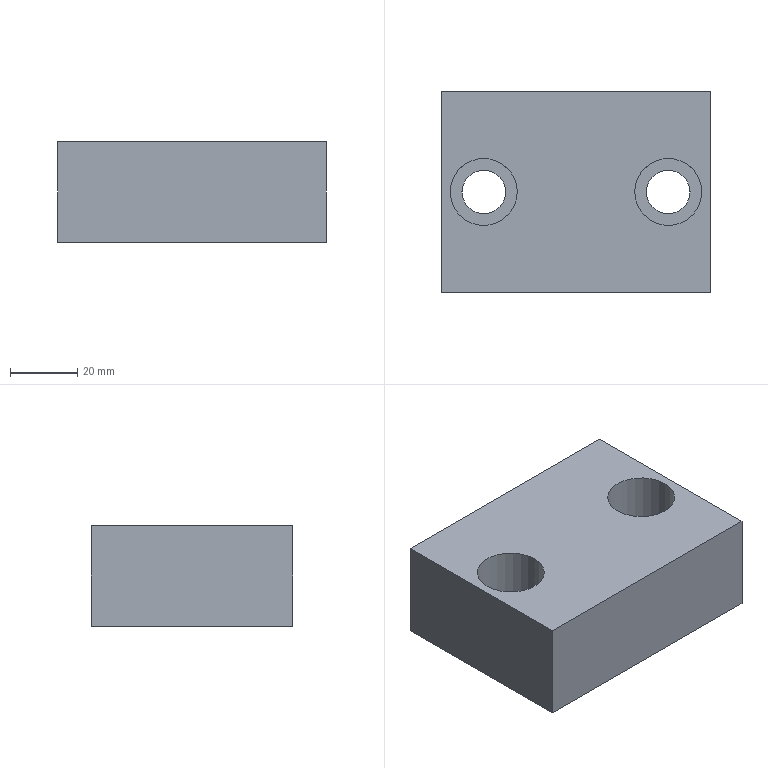Part | NX | features solid 2 | 1 solid | 12 faces | box 80 x 60 x 30 mm | volume 130956 mm3 | plane 8 | cylinder 4 | commonest cylinder face diameters 13 x2 20 x2
STEP:
#1=CARTESIAN_POINT('',(955.,365.,2.));
#2=VERTEX_POINT('',#1);
#3=CARTESIAN_POINT('',(955.,425.,2.));
#4=VERTEX_POINT('',#3);
#5=CARTESIAN_POINT('',(955.,365.,2.));
#6=DIRECTION('',(0.,1.,0.));
#7=VECTOR('',#6,1000.);
#8=LINE('',#5,#7);
#9=EDGE_CURVE('',#2,#4,#8,.T.);
#10=ORIENTED_EDGE('',*,*,#9,.F.);
#11=CARTESIAN_POINT('',(1035.,365.,2.));
#12=VERTEX_POINT('',#11);
#13=CARTESIAN_POINT('',(1035.,365.,2.));
#14=DIRECTION('',(-1.,0.,0.));
#15=VECTOR('',#14,1000.);
#16=LINE('',#13,#15);
#17=EDGE_CURVE('',#12,#2,#16,.T.);
#18=ORIENTED_EDGE('',*,*,#17,.F.);
#19=CARTESIAN_POINT('',(1035.,425.,2.));
#20=VERTEX_POINT('',#19);
#21=CARTESIAN_POINT('',(1035.,425.,2.));
#22=DIRECTION('',(0.,-1.,0.));
#23=VECTOR('',#22,1000.);
#24=LINE('',#21,#23);
#25=EDGE_CURVE('',#20,#12,#24,.T.);
#26=ORIENTED_EDGE('',*,*,#25,.F.);
#27=CARTESIAN_POINT('',(955.,425.,2.));
#28=DIRECTION('',(1.,0.,0.));
#29=VECTOR('',#28,1000.);
#30=LINE('',#27,#29);
#31=EDGE_CURVE('',#4,#20,#30,.T.);
#32=ORIENTED_EDGE('',*,*,#31,.F.);
#33=EDGE_LOOP('',(#10,#18,#26,#32));
#34=FACE_BOUND('',#33,.T.);
#35=CARTESIAN_POINT('',(1012.5,395.,2.));
#36=VERTEX_POINT('',#35);
#37=CARTESIAN_POINT('',(1022.5,395.,2.));
#38=DIRECTION('',(0.,0.,-1.));
#39=DIRECTION('',(-1.,0.,0.));
#40=AXIS2_PLACEMENT_3D('',#37,#38,#39);
#41=CIRCLE('',#40,10.);
#42=EDGE_CURVE('',#36,#36,#41,.T.);
#43=ORIENTED_EDGE('',*,*,#42,.T.);
#44=EDGE_LOOP('',(#43));
#45=FACE_BOUND('',#44,.T.);
#46=CARTESIAN_POINT('',(977.5,395.,2.));
#47=VERTEX_POINT('',#46);
#48=CARTESIAN_POINT('',(967.5,395.,2.));
#49=DIRECTION('',(0.,0.,1.));
#50=DIRECTION('',(1.,0.,0.));
#51=AXIS2_PLACEMENT_3D('',#48,#49,#50);
#52=CIRCLE('',#51,10.);
#53=EDGE_CURVE('',#47,#47,#52,.T.);
#54=ORIENTED_EDGE('',*,*,#53,.F.);
#55=EDGE_LOOP('',(#54));
#56=FACE_BOUND('',#55,.T.);
#57=CARTESIAN_POINT('',(955.,365.,2.));
#58=DIRECTION('',(0.,0.,1.));
#59=DIRECTION('',(1.,0.,0.));
#60=AXIS2_PLACEMENT_3D('',#57,#58,#59);
#61=PLANE('',#60);
#62=ADVANCED_FACE('',(#34,#45,#56),#61,.T.);
#63=CARTESIAN_POINT('',(974.,395.,-28.));
#64=VERTEX_POINT('',#63);
#65=CARTESIAN_POINT('',(967.5,395.,-28.));
#66=DIRECTION('',(0.,0.,1.));
#67=DIRECTION('',(1.,0.,0.));
#68=AXIS2_PLACEMENT_3D('',#65,#66,#67);
#69=CIRCLE('',#68,6.5);
#70=EDGE_CURVE('',#64,#64,#69,.T.);
#71=ORIENTED_EDGE('',*,*,#70,.F.);
#72=EDGE_LOOP('',(#71));
#73=FACE_BOUND('',#72,.T.);
#74=CARTESIAN_POINT('',(974.,395.,-12.));
#75=VERTEX_POINT('',#74);
#76=CARTESIAN_POINT('',(967.5,395.,-12.));
#77=DIRECTION('',(0.,0.,1.));
#78=DIRECTION('',(1.,0.,0.));
#79=AXIS2_PLACEMENT_3D('',#76,#77,#78);
#80=CIRCLE('',#79,6.5);
#81=EDGE_CURVE('',#75,#75,#80,.T.);
#82=ORIENTED_EDGE('',*,*,#81,.T.);
#83=EDGE_LOOP('',(#82));
#84=FACE_BOUND('',#83,.T.);
#85=CARTESIAN_POINT('',(967.5,395.,2.));
#86=DIRECTION('',(0.,0.,-1.));
#87=DIRECTION('',(-1.,0.,0.));
#88=AXIS2_PLACEMENT_3D('',#85,#86,#87);
#89=CYLINDRICAL_SURFACE('',#88,6.5);
#90=ADVANCED_FACE('',(#73,#84),#89,.F.);
#91=CARTESIAN_POINT('',(955.,365.,-28.));
#92=VERTEX_POINT('',#91);
#93=CARTESIAN_POINT('',(955.,425.,-28.));
#94=VERTEX_POINT('',#93);
#95=CARTESIAN_POINT('',(955.,365.,-28.));
#96=DIRECTION('',(0.,1.,0.));
#97=VECTOR('',#96,1000.);
#98=LINE('',#95,#97);
#99=EDGE_CURVE('',#92,#94,#98,.T.);
#100=ORIENTED_EDGE('',*,*,#99,.T.);
#101=CARTESIAN_POINT('',(1035.,425.,-28.));
#102=VERTEX_POINT('',#101);
#103=CARTESIAN_POINT('',(955.,425.,-28.));
#104=DIRECTION('',(1.,0.,0.));
#105=VECTOR('',#104,1000.);
#106=LINE('',#103,#105);
#107=EDGE_CURVE('',#94,#102,#106,.T.);
#108=ORIENTED_EDGE('',*,*,#107,.T.);
#109=CARTESIAN_POINT('',(1035.,365.,-28.));
#110=VERTEX_POINT('',#109);
#111=CARTESIAN_POINT('',(1035.,425.,-28.));
#112=DIRECTION('',(0.,-1.,0.));
#113=VECTOR('',#112,1000.);
#114=LINE('',#111,#113);
#115=EDGE_CURVE('',#102,#110,#114,.T.);
#116=ORIENTED_EDGE('',*,*,#115,.T.);
#117=CARTESIAN_POINT('',(1035.,365.,-28.));
#118=DIRECTION('',(-1.,0.,0.));
#119=VECTOR('',#118,1000.);
#120=LINE('',#117,#119);
#121=EDGE_CURVE('',#110,#92,#120,.T.);
#122=ORIENTED_EDGE('',*,*,#121,.T.);
#123=EDGE_LOOP('',(#100,#108,#116,#122));
#124=FACE_BOUND('',#123,.T.);
#125=CARTESIAN_POINT('',(1029.,395.,-28.));
#126=VERTEX_POINT('',#125);
#127=CARTESIAN_POINT('',(1022.5,395.,-28.));
#128=DIRECTION('',(0.,0.,1.));
#129=DIRECTION('',(1.,0.,0.));
#130=AXIS2_PLACEMENT_3D('',#127,#128,#129);
#131=CIRCLE('',#130,6.5);
#132=EDGE_CURVE('',#126,#126,#131,.F.);
#133=ORIENTED_EDGE('',*,*,#132,.F.);
#134=EDGE_LOOP('',(#133));
#135=FACE_BOUND('',#134,.T.);
#136=ORIENTED_EDGE('',*,*,#70,.T.);
#137=EDGE_LOOP('',(#136));
#138=FACE_BOUND('',#137,.T.);
#139=CARTESIAN_POINT('',(955.,365.,-28.));
#140=DIRECTION('',(0.,0.,1.));
#141=DIRECTION('',(1.,0.,0.));
#142=AXIS2_PLACEMENT_3D('',#139,#140,#141);
#143=PLANE('',#142);
#144=ADVANCED_FACE('',(#124,#135,#138),#143,.F.);
#145=ORIENTED_EDGE('',*,*,#99,.F.);
#146=CARTESIAN_POINT('',(955.,365.,2.));
#147=DIRECTION('',(0.,0.,-1.));
#148=VECTOR('',#147,1000.);
#149=LINE('',#146,#148);
#150=EDGE_CURVE('',#2,#92,#149,.T.);
#151=ORIENTED_EDGE('',*,*,#150,.F.);
#152=ORIENTED_EDGE('',*,*,#9,.T.);
#153=CARTESIAN_POINT('',(955.,425.,2.));
#154=DIRECTION('',(0.,0.,-1.));
#155=VECTOR('',#154,1000.);
#156=LINE('',#153,#155);
#157=EDGE_CURVE('',#4,#94,#156,.T.);
#158=ORIENTED_EDGE('',*,*,#157,.T.);
#159=EDGE_LOOP('',(#145,#151,#152,#158));
#160=FACE_BOUND('',#159,.T.);
#161=CARTESIAN_POINT('',(955.,365.,2.));
#162=DIRECTION('',(-1.,0.,0.));
#163=DIRECTION('',(0.,-1.,0.));
#164=AXIS2_PLACEMENT_3D('',#161,#162,#163);
#165=PLANE('',#164);
#166=ADVANCED_FACE('',(#160),#165,.T.);
#167=ORIENTED_EDGE('',*,*,#107,.F.);
#168=ORIENTED_EDGE('',*,*,#157,.F.);
#169=ORIENTED_EDGE('',*,*,#31,.T.);
#170=CARTESIAN_POINT('',(1035.,425.,2.));
#171=DIRECTION('',(0.,0.,-1.));
#172=VECTOR('',#171,1000.);
#173=LINE('',#170,#172);
#174=EDGE_CURVE('',#20,#102,#173,.T.);
#175=ORIENTED_EDGE('',*,*,#174,.T.);
#176=EDGE_LOOP('',(#167,#168,#169,#175));
#177=FACE_BOUND('',#176,.T.);
#178=CARTESIAN_POINT('',(955.,425.,2.));
#179=DIRECTION('',(0.,1.,0.));
#180=DIRECTION('',(0.,0.,1.));
#181=AXIS2_PLACEMENT_3D('',#178,#179,#180);
#182=PLANE('',#181);
#183=ADVANCED_FACE('',(#177),#182,.T.);
#184=ORIENTED_EDGE('',*,*,#115,.F.);
#185=ORIENTED_EDGE('',*,*,#174,.F.);
#186=ORIENTED_EDGE('',*,*,#25,.T.);
#187=CARTESIAN_POINT('',(1035.,365.,2.));
#188=DIRECTION('',(0.,0.,-1.));
#189=VECTOR('',#188,1000.);
#190=LINE('',#187,#189);
#191=EDGE_CURVE('',#12,#110,#190,.T.);
#192=ORIENTED_EDGE('',*,*,#191,.T.);
#193=EDGE_LOOP('',(#184,#185,#186,#192));
#194=FACE_BOUND('',#193,.T.);
#195=CARTESIAN_POINT('',(1035.,425.,2.));
#196=DIRECTION('',(1.,0.,0.));
#197=DIRECTION('',(0.,1.,0.));
#198=AXIS2_PLACEMENT_3D('',#195,#196,#197);
#199=PLANE('',#198);
#200=ADVANCED_FACE('',(#194),#199,.T.);
#201=ORIENTED_EDGE('',*,*,#121,.F.);
#202=ORIENTED_EDGE('',*,*,#191,.F.);
#203=ORIENTED_EDGE('',*,*,#17,.T.);
#204=ORIENTED_EDGE('',*,*,#150,.T.);
#205=EDGE_LOOP('',(#201,#202,#203,#204));
#206=FACE_BOUND('',#205,.T.);
#207=CARTESIAN_POINT('',(1035.,365.,2.));
#208=DIRECTION('',(0.,-1.,0.));
#209=DIRECTION('',(1.,0.,0.));
#210=AXIS2_PLACEMENT_3D('',#207,#208,#209);
#211=PLANE('',#210);
#212=ADVANCED_FACE('',(#206),#211,.T.);
#213=CARTESIAN_POINT('',(1016.,395.,-12.));
#214=VERTEX_POINT('',#213);
#215=CARTESIAN_POINT('',(1022.5,395.,-12.));
#216=DIRECTION('',(0.,0.,-1.));
#217=DIRECTION('',(-1.,0.,0.));
#218=AXIS2_PLACEMENT_3D('',#215,#216,#217);
#219=CIRCLE('',#218,6.5);
#220=EDGE_CURVE('',#214,#214,#219,.F.);
#221=ORIENTED_EDGE('',*,*,#220,.T.);
#222=EDGE_LOOP('',(#221));
#223=FACE_BOUND('',#222,.T.);
#224=ORIENTED_EDGE('',*,*,#132,.T.);
#225=EDGE_LOOP('',(#224));
#226=FACE_BOUND('',#225,.T.);
#227=CARTESIAN_POINT('',(1022.5,395.,2.));
#228=DIRECTION('',(0.,0.,-1.));
#229=DIRECTION('',(-1.,0.,0.));
#230=AXIS2_PLACEMENT_3D('',#227,#228,#229);
#231=CYLINDRICAL_SURFACE('',#230,6.5);
#232=ADVANCED_FACE('',(#223,#226),#231,.F.);
#233=CARTESIAN_POINT('',(1012.5,395.,-12.));
#234=VERTEX_POINT('',#233);
#235=CARTESIAN_POINT('',(1022.5,395.,-12.));
#236=DIRECTION('',(0.,0.,-1.));
#237=DIRECTION('',(-1.,0.,0.));
#238=AXIS2_PLACEMENT_3D('',#235,#236,#237);
#239=CIRCLE('',#238,10.);
#240=EDGE_CURVE('',#234,#234,#239,.T.);
#241=ORIENTED_EDGE('',*,*,#240,.F.);
#242=EDGE_LOOP('',(#241));
#243=FACE_BOUND('',#242,.T.);
#244=ORIENTED_EDGE('',*,*,#220,.F.);
#245=EDGE_LOOP('',(#244));
#246=FACE_BOUND('',#245,.T.);
#247=CARTESIAN_POINT('',(1022.5,395.,-12.));
#248=DIRECTION('',(0.,0.,-1.));
#249=DIRECTION('',(-1.,0.,0.));
#250=AXIS2_PLACEMENT_3D('',#247,#248,#249);
#251=PLANE('',#250);
#252=ADVANCED_FACE('',(#243,#246),#251,.F.);
#253=ORIENTED_EDGE('',*,*,#42,.F.);
#254=EDGE_LOOP('',(#253));
#255=FACE_BOUND('',#254,.T.);
#256=ORIENTED_EDGE('',*,*,#240,.T.);
#257=EDGE_LOOP('',(#256));
#258=FACE_BOUND('',#257,.T.);
#259=CARTESIAN_POINT('',(1022.5,395.,2.));
#260=DIRECTION('',(0.,0.,-1.));
#261=DIRECTION('',(-1.,0.,0.));
#262=AXIS2_PLACEMENT_3D('',#259,#260,#261);
#263=CYLINDRICAL_SURFACE('',#262,10.);
#264=ADVANCED_FACE('',(#255,#258),#263,.F.);
#265=ORIENTED_EDGE('',*,*,#53,.T.);
#266=EDGE_LOOP('',(#265));
#267=FACE_BOUND('',#266,.T.);
#268=CARTESIAN_POINT('',(977.5,395.,-12.));
#269=VERTEX_POINT('',#268);
#270=CARTESIAN_POINT('',(967.5,395.,-12.));
#271=DIRECTION('',(0.,0.,1.));
#272=DIRECTION('',(1.,0.,0.));
#273=AXIS2_PLACEMENT_3D('',#270,#271,#272);
#274=CIRCLE('',#273,10.);
#275=EDGE_CURVE('',#269,#269,#274,.T.);
#276=ORIENTED_EDGE('',*,*,#275,.F.);
#277=EDGE_LOOP('',(#276));
#278=FACE_BOUND('',#277,.T.);
#279=CARTESIAN_POINT('',(967.5,395.,2.));
#280=DIRECTION('',(0.,0.,-1.));
#281=DIRECTION('',(-1.,0.,0.));
#282=AXIS2_PLACEMENT_3D('',#279,#280,#281);
#283=CYLINDRICAL_SURFACE('',#282,10.);
#284=ADVANCED_FACE('',(#267,#278),#283,.F.);
#285=ORIENTED_EDGE('',*,*,#81,.F.);
#286=EDGE_LOOP('',(#285));
#287=FACE_BOUND('',#286,.T.);
#288=ORIENTED_EDGE('',*,*,#275,.T.);
#289=EDGE_LOOP('',(#288));
#290=FACE_BOUND('',#289,.T.);
#291=CARTESIAN_POINT('',(967.5,395.,-12.));
#292=DIRECTION('',(0.,0.,1.));
#293=DIRECTION('',(1.,0.,0.));
#294=AXIS2_PLACEMENT_3D('',#291,#292,#293);
#295=PLANE('',#294);
#296=ADVANCED_FACE('',(#287,#290),#295,.T.);
#297=CLOSED_SHELL('',(#62,#90,#144,#166,#183,#200,#212,#232,#252,#264,#284,#296));
#298=MANIFOLD_SOLID_BREP('',#297);
#299=(LENGTH_UNIT()NAMED_UNIT(*)SI_UNIT(.MILLI.,.METRE.));
#300=UNCERTAINTY_MEASURE_WITH_UNIT(LENGTH_MEASURE(0.00001),#299,'','');
#301=(NAMED_UNIT(*)PLANE_ANGLE_UNIT()SI_UNIT($,.RADIAN.));
#302=(NAMED_UNIT(*)SI_UNIT($,.STERADIAN.)SOLID_ANGLE_UNIT());
#303=(GEOMETRIC_REPRESENTATION_CONTEXT(3)GLOBAL_UNCERTAINTY_ASSIGNED_CONTEXT((#300))GLOBAL_UNIT_ASSIGNED_CONTEXT((#299,#301,#302))REPRESENTATION_CONTEXT('',''));
#304=ADVANCED_BREP_SHAPE_REPRESENTATION('',(#298),#303);